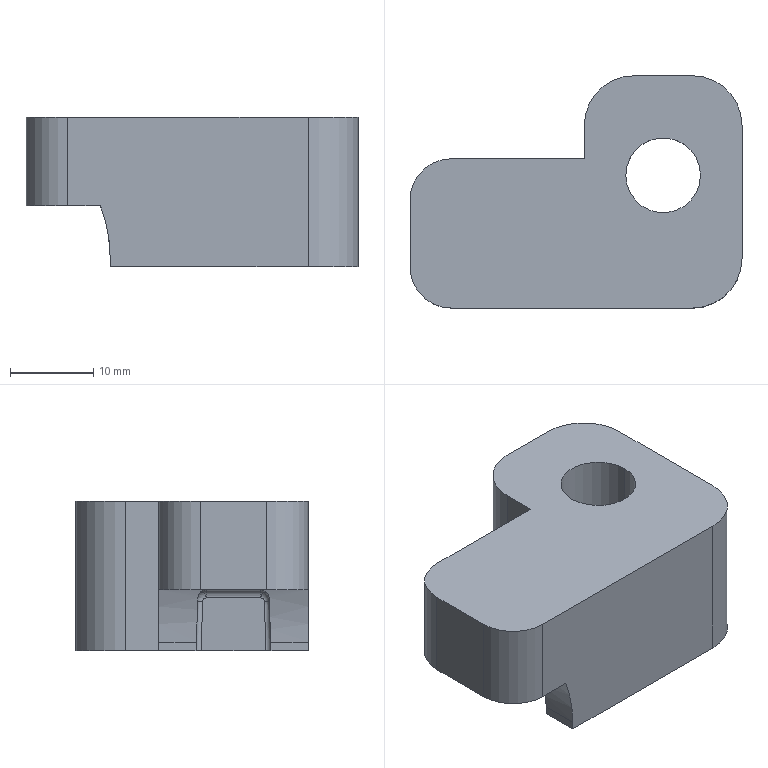Part | Creo | 1 solid | 157 faces | box 40 x 28 x 18 mm | volume 12165 mm3 | other 86 | plane 44 | cylinder 23 | spline 2 | sphere 2 | commonest cylinder face diameters 2.008 x3 12 x3 1.044 x2 1.205 x2 9 x2 10 x2